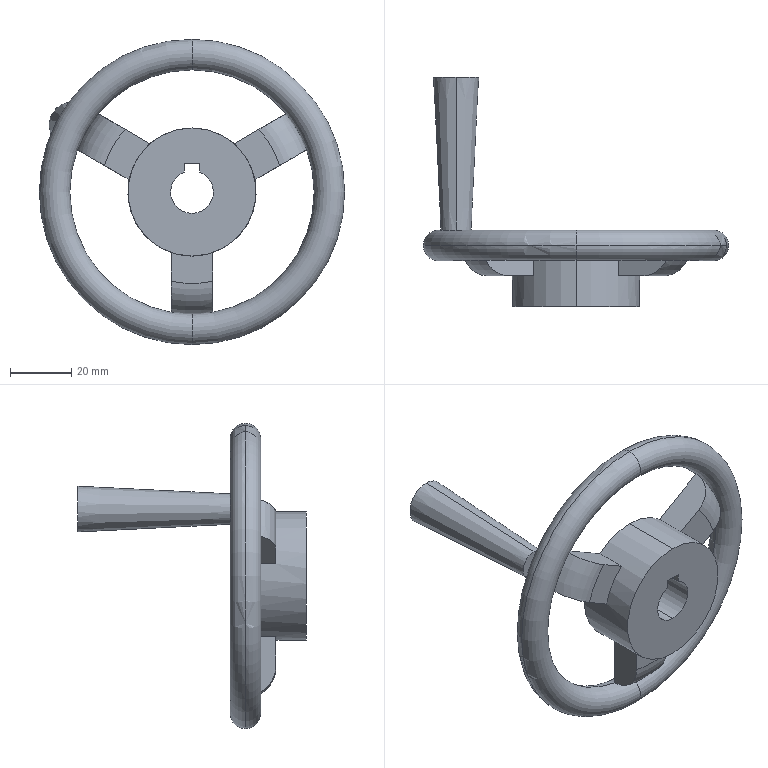Part | SolidWorks | features ICE 4, 3DProfileFeature 1, Fillet 1, Revolution 1, Sweep 1 | 3 solids | 29 faces | box 100 x 75 x 100 mm | volume 59765 mm3 | plane 16 | torus 7 | cylinder 4 | cone 2 | commonest cylinder face diameters 14 x2 42 x2
STEP:
#1=CARTESIAN_POINT('',(0.,0.,-50.));
#2=VERTEX_POINT('',#1);
#3=CARTESIAN_POINT('',(0.,0.,-40.));
#4=VERTEX_POINT('',#3);
#5=CARTESIAN_POINT('',(0.,0.,-45.));
#6=DIRECTION('',(1.,0.,0.));
#7=DIRECTION('',(0.,0.,-1.));
#8=AXIS2_PLACEMENT_3D('',#5,#6,#7);
#9=CIRCLE('',#8,5.);
#10=EDGE_CURVE('',#2,#4,#9,.T.);
#11=ORIENTED_EDGE('',*,*,#10,.F.);
#12=CARTESIAN_POINT('',(0.,0.,50.));
#13=VERTEX_POINT('',#12);
#14=CARTESIAN_POINT('',(0.,0.,0.));
#15=DIRECTION('',(0.,1.,0.));
#16=DIRECTION('',(0.,0.,1.));
#17=AXIS2_PLACEMENT_3D('',#14,#15,#16);
#18=CIRCLE('',#17,50.);
#19=EDGE_CURVE('',#2,#13,#18,.T.);
#20=ORIENTED_EDGE('',*,*,#19,.T.);
#21=CARTESIAN_POINT('',(0.,0.,40.));
#22=VERTEX_POINT('',#21);
#23=CARTESIAN_POINT('',(0.,0.,45.));
#24=DIRECTION('',(-1.,0.,0.));
#25=DIRECTION('',(0.,0.,1.));
#26=AXIS2_PLACEMENT_3D('',#23,#24,#25);
#27=CIRCLE('',#26,5.);
#28=EDGE_CURVE('',#13,#22,#27,.T.);
#29=ORIENTED_EDGE('',*,*,#28,.T.);
#30=CARTESIAN_POINT('',(0.,0.,0.));
#31=DIRECTION('',(0.,1.,0.));
#32=DIRECTION('',(0.,0.,1.));
#33=AXIS2_PLACEMENT_3D('',#30,#31,#32);
#34=CIRCLE('',#33,40.);
#35=EDGE_CURVE('',#4,#22,#34,.T.);
#36=ORIENTED_EDGE('',*,*,#35,.F.);
#37=EDGE_LOOP('',(#11,#20,#29,#36));
#38=FACE_OUTER_BOUND('',#37,.T.);
#39=CARTESIAN_POINT('',(0.,0.,0.));
#40=DIRECTION('',(0.,1.,0.));
#41=DIRECTION('',(0.,0.,1.));
#42=AXIS2_PLACEMENT_3D('',#39,#40,#41);
#43=TOROIDAL_SURFACE('',#42,45.,5.);
#44=ADVANCED_FACE('',(#38),#43,.T.);
#45=ORIENTED_EDGE('',*,*,#28,.F.);
#46=CARTESIAN_POINT('',(0.,0.,0.));
#47=DIRECTION('',(0.,1.,0.));
#48=DIRECTION('',(0.,0.,1.));
#49=AXIS2_PLACEMENT_3D('',#46,#47,#48);
#50=CIRCLE('',#49,50.);
#51=EDGE_CURVE('',#13,#2,#50,.T.);
#52=ORIENTED_EDGE('',*,*,#51,.T.);
#53=ORIENTED_EDGE('',*,*,#10,.T.);
#54=CARTESIAN_POINT('',(0.,0.,0.));
#55=DIRECTION('',(0.,1.,0.));
#56=DIRECTION('',(0.,0.,1.));
#57=AXIS2_PLACEMENT_3D('',#54,#55,#56);
#58=CIRCLE('',#57,40.);
#59=EDGE_CURVE('',#22,#4,#58,.T.);
#60=ORIENTED_EDGE('',*,*,#59,.F.);
#61=EDGE_LOOP('',(#45,#52,#53,#60));
#62=FACE_OUTER_BOUND('',#61,.T.);
#63=CARTESIAN_POINT('',(0.,0.,0.));
#64=DIRECTION('',(0.,1.,0.));
#65=DIRECTION('',(0.,0.,1.));
#66=AXIS2_PLACEMENT_3D('',#63,#64,#65);
#67=TOROIDAL_SURFACE('',#66,45.,5.);
#68=ADVANCED_FACE('',(#62),#67,.T.);
#69=ORIENTED_EDGE('',*,*,#51,.F.);
#70=CARTESIAN_POINT('',(0.,0.,45.));
#71=DIRECTION('',(-1.,0.,0.));
#72=DIRECTION('',(0.,0.,1.));
#73=AXIS2_PLACEMENT_3D('',#70,#71,#72);
#74=CIRCLE('',#73,5.);
#75=EDGE_CURVE('',#22,#13,#74,.T.);
#76=ORIENTED_EDGE('',*,*,#75,.F.);
#77=ORIENTED_EDGE('',*,*,#59,.T.);
#78=CARTESIAN_POINT('',(0.,0.,-45.));
#79=DIRECTION('',(1.,0.,0.));
#80=DIRECTION('',(0.,0.,-1.));
#81=AXIS2_PLACEMENT_3D('',#78,#79,#80);
#82=CIRCLE('',#81,5.);
#83=EDGE_CURVE('',#4,#2,#82,.T.);
#84=ORIENTED_EDGE('',*,*,#83,.T.);
#85=EDGE_LOOP('',(#69,#76,#77,#84));
#86=FACE_OUTER_BOUND('',#85,.T.);
#87=CARTESIAN_POINT('',(0.,0.,0.));
#88=DIRECTION('',(0.,1.,0.));
#89=DIRECTION('',(0.,0.,1.));
#90=AXIS2_PLACEMENT_3D('',#87,#88,#89);
#91=TOROIDAL_SURFACE('',#90,45.,5.);
#92=ADVANCED_FACE('',(#86),#91,.T.);
#93=ORIENTED_EDGE('',*,*,#19,.F.);
#94=ORIENTED_EDGE('',*,*,#83,.F.);
#95=ORIENTED_EDGE('',*,*,#35,.T.);
#96=ORIENTED_EDGE('',*,*,#75,.T.);
#97=EDGE_LOOP('',(#93,#94,#95,#96));
#98=FACE_OUTER_BOUND('',#97,.T.);
#99=CARTESIAN_POINT('',(0.,0.,0.));
#100=DIRECTION('',(0.,1.,0.));
#101=DIRECTION('',(0.,0.,1.));
#102=AXIS2_PLACEMENT_3D('',#99,#100,#101);
#103=TOROIDAL_SURFACE('',#102,45.,5.);
#104=ADVANCED_FACE('',(#98),#103,.T.);
#105=CLOSED_SHELL('',(#44,#68,#92,#104));
#106=MANIFOLD_SOLID_BREP('',#105);
#107=CARTESIAN_POINT('',(-39.297,5.,16.925));
#108=VERTEX_POINT('',#107);
#109=CARTESIAN_POINT('',(-39.297,5.,26.925));
#110=VERTEX_POINT('',#109);
#111=CARTESIAN_POINT('',(-39.297,5.,21.925));
#112=DIRECTION('',(0.,-1.,0.));
#113=DIRECTION('',(0.,0.,-1.));
#114=AXIS2_PLACEMENT_3D('',#111,#112,#113);
#115=CIRCLE('',#114,5.);
#116=EDGE_CURVE('',#108,#110,#115,.T.);
#117=ORIENTED_EDGE('',*,*,#116,.F.);
#118=CARTESIAN_POINT('',(-39.297,55.,14.425));
#119=VERTEX_POINT('',#118);
#120=CARTESIAN_POINT('',(-39.297,55.,14.425));
#121=DIRECTION('',(0.,0.9988,-0.04994));
#122=VECTOR('',#121,1000.);
#123=LINE('',#120,#122);
#124=EDGE_CURVE('',#108,#119,#123,.T.);
#125=ORIENTED_EDGE('',*,*,#124,.T.);
#126=CARTESIAN_POINT('',(-39.297,55.,29.425));
#127=VERTEX_POINT('',#126);
#128=CARTESIAN_POINT('',(-39.297,55.,21.925));
#129=DIRECTION('',(0.,-1.,0.));
#130=DIRECTION('',(0.,0.,-1.));
#131=AXIS2_PLACEMENT_3D('',#128,#129,#130);
#132=CIRCLE('',#131,7.5);
#133=EDGE_CURVE('',#119,#127,#132,.T.);
#134=ORIENTED_EDGE('',*,*,#133,.T.);
#135=CARTESIAN_POINT('',(-39.297,55.,29.425));
#136=DIRECTION('',(0.,0.9988,0.04994));
#137=VECTOR('',#136,1000.);
#138=LINE('',#135,#137);
#139=EDGE_CURVE('',#110,#127,#138,.T.);
#140=ORIENTED_EDGE('',*,*,#139,.F.);
#141=EDGE_LOOP('',(#117,#125,#134,#140));
#142=FACE_OUTER_BOUND('',#141,.T.);
#143=CARTESIAN_POINT('',(-39.297,55.,21.925));
#144=DIRECTION('',(0.,1.,0.));
#145=DIRECTION('',(0.,0.,1.));
#146=AXIS2_PLACEMENT_3D('',#143,#144,#145);
#147=CONICAL_SURFACE('',#146,7.5,0.04996);
#148=ADVANCED_FACE('',(#142),#147,.T.);
#149=ORIENTED_EDGE('',*,*,#124,.F.);
#150=CARTESIAN_POINT('',(-39.297,5.,21.925));
#151=DIRECTION('',(0.,-1.,0.));
#152=DIRECTION('',(0.,0.,-1.));
#153=AXIS2_PLACEMENT_3D('',#150,#151,#152);
#154=CIRCLE('',#153,5.);
#155=EDGE_CURVE('',#110,#108,#154,.T.);
#156=ORIENTED_EDGE('',*,*,#155,.F.);
#157=ORIENTED_EDGE('',*,*,#139,.T.);
#158=CARTESIAN_POINT('',(-39.297,55.,21.925));
#159=DIRECTION('',(0.,-1.,0.));
#160=DIRECTION('',(0.,0.,-1.));
#161=AXIS2_PLACEMENT_3D('',#158,#159,#160);
#162=CIRCLE('',#161,7.5);
#163=EDGE_CURVE('',#127,#119,#162,.T.);
#164=ORIENTED_EDGE('',*,*,#163,.T.);
#165=EDGE_LOOP('',(#149,#156,#157,#164));
#166=FACE_OUTER_BOUND('',#165,.T.);
#167=CARTESIAN_POINT('',(-39.297,55.,21.925));
#168=DIRECTION('',(0.,1.,0.));
#169=DIRECTION('',(0.,0.,1.));
#170=AXIS2_PLACEMENT_3D('',#167,#168,#169);
#171=CONICAL_SURFACE('',#170,7.5,0.04996);
#172=ADVANCED_FACE('',(#166),#171,.T.);
#173=ORIENTED_EDGE('',*,*,#155,.T.);
#174=ORIENTED_EDGE('',*,*,#116,.T.);
#175=EDGE_LOOP('',(#173,#174));
#176=FACE_OUTER_BOUND('',#175,.T.);
#177=CARTESIAN_POINT('',(-39.297,5.,0.));
#178=DIRECTION('',(0.,1.,0.));
#179=DIRECTION('',(0.,0.,1.));
#180=AXIS2_PLACEMENT_3D('',#177,#178,#179);
#181=PLANE('',#180);
#182=ADVANCED_FACE('',(#176),#181,.F.);
#183=ORIENTED_EDGE('',*,*,#163,.F.);
#184=ORIENTED_EDGE('',*,*,#133,.F.);
#185=EDGE_LOOP('',(#183,#184));
#186=FACE_OUTER_BOUND('',#185,.T.);
#187=CARTESIAN_POINT('',(-39.297,55.,0.));
#188=DIRECTION('',(0.,-1.,0.));
#189=DIRECTION('',(0.,0.,-1.));
#190=AXIS2_PLACEMENT_3D('',#187,#188,#189);
#191=PLANE('',#190);
#192=ADVANCED_FACE('',(#186),#191,.F.);
#193=CLOSED_SHELL('',(#148,#172,#182,#192));
#194=MANIFOLD_SOLID_BREP('',#193);
#195=CARTESIAN_POINT('',(2.5,0.,6.538));
#196=VERTEX_POINT('',#195);
#197=CARTESIAN_POINT('',(0.,0.,-7.));
#198=VERTEX_POINT('',#197);
#199=CARTESIAN_POINT('',(0.,0.,0.));
#200=DIRECTION('',(0.,1.,0.));
#201=DIRECTION('',(0.,0.,1.));
#202=AXIS2_PLACEMENT_3D('',#199,#200,#201);
#203=CIRCLE('',#202,7.);
#204=EDGE_CURVE('',#196,#198,#203,.T.);
#205=ORIENTED_EDGE('',*,*,#204,.T.);
#206=CARTESIAN_POINT('',(0.,-20.,-7.));
#207=VERTEX_POINT('',#206);
#208=CARTESIAN_POINT('',(0.,55.,-7.));
#209=DIRECTION('',(0.,-1.,0.));
#210=VECTOR('',#209,1000.);
#211=LINE('',#208,#210);
#212=EDGE_CURVE('',#198,#207,#211,.T.);
#213=ORIENTED_EDGE('',*,*,#212,.T.);
#214=CARTESIAN_POINT('',(2.5,-20.,6.538));
#215=VERTEX_POINT('',#214);
#216=CARTESIAN_POINT('',(0.,-20.,0.));
#217=DIRECTION('',(0.,-1.,0.));
#218=DIRECTION('',(0.,0.,-1.));
#219=AXIS2_PLACEMENT_3D('',#216,#217,#218);
#220=CIRCLE('',#219,7.);
#221=EDGE_CURVE('',#207,#215,#220,.T.);
#222=ORIENTED_EDGE('',*,*,#221,.T.);
#223=CARTESIAN_POINT('',(2.5,55.,6.538));
#224=DIRECTION('',(0.,1.,0.));
#225=VECTOR('',#224,1000.);
#226=LINE('',#223,#225);
#227=EDGE_CURVE('',#215,#196,#226,.T.);
#228=ORIENTED_EDGE('',*,*,#227,.T.);
#229=EDGE_LOOP('',(#205,#213,#222,#228));
#230=FACE_OUTER_BOUND('',#229,.T.);
#231=CARTESIAN_POINT('',(0.,55.,0.));
#232=DIRECTION('',(0.,-1.,0.));
#233=DIRECTION('',(0.,0.,-1.));
#234=AXIS2_PLACEMENT_3D('',#231,#232,#233);
#235=CYLINDRICAL_SURFACE('',#234,7.);
#236=ADVANCED_FACE('',(#230),#235,.F.);
#237=CARTESIAN_POINT('',(0.,-20.,-21.));
#238=VERTEX_POINT('',#237);
#239=CARTESIAN_POINT('',(0.,-20.,21.));
#240=VERTEX_POINT('',#239);
#241=CARTESIAN_POINT('',(0.,-20.,0.));
#242=DIRECTION('',(0.,-1.,0.));
#243=DIRECTION('',(0.,0.,-1.));
#244=AXIS2_PLACEMENT_3D('',#241,#242,#243);
#245=CIRCLE('',#244,21.);
#246=EDGE_CURVE('',#238,#240,#245,.T.);
#247=ORIENTED_EDGE('',*,*,#246,.F.);
#248=CARTESIAN_POINT('',(0.,-10.,-21.));
#249=VERTEX_POINT('',#248);
#250=CARTESIAN_POINT('',(0.,-10.,-21.));
#251=DIRECTION('',(0.,1.,0.));
#252=VECTOR('',#251,1000.);
#253=LINE('',#250,#252);
#254=EDGE_CURVE('',#238,#249,#253,.T.);
#255=ORIENTED_EDGE('',*,*,#254,.T.);
#256=CARTESIAN_POINT('',(6.811,-10.,-19.865));
#257=VERTEX_POINT('',#256);
#258=CARTESIAN_POINT('',(0.,-10.,0.));
#259=DIRECTION('',(0.,-1.,0.));
#260=DIRECTION('',(0.,0.,1.));
#261=AXIS2_PLACEMENT_3D('',#258,#259,#260);
#262=CIRCLE('',#261,21.);
#263=EDGE_CURVE('',#249,#257,#262,.T.);
#264=ORIENTED_EDGE('',*,*,#263,.T.);
#265=CARTESIAN_POINT('',(6.811,0.,-19.865));
#266=VERTEX_POINT('',#265);
#267=CARTESIAN_POINT('',(6.811,-10.,-19.865));
#268=DIRECTION('',(0.,1.,0.));
#269=VECTOR('',#268,1000.);
#270=LINE('',#267,#269);
#271=EDGE_CURVE('',#257,#266,#270,.T.);
#272=ORIENTED_EDGE('',*,*,#271,.T.);
#273=CARTESIAN_POINT('',(20.609,0.,4.034));
#274=VERTEX_POINT('',#273);
#275=CARTESIAN_POINT('',(0.,0.,0.));
#276=DIRECTION('',(0.,1.,0.));
#277=DIRECTION('',(0.,0.,1.));
#278=AXIS2_PLACEMENT_3D('',#275,#276,#277);
#279=CIRCLE('',#278,21.);
#280=EDGE_CURVE('',#274,#266,#279,.T.);
#281=ORIENTED_EDGE('',*,*,#280,.F.);
#282=CARTESIAN_POINT('',(20.609,-10.,4.034));
#283=VERTEX_POINT('',#282);
#284=CARTESIAN_POINT('',(20.609,-10.,4.034));
#285=DIRECTION('',(0.,1.,0.));
#286=VECTOR('',#285,1000.);
#287=LINE('',#284,#286);
#288=EDGE_CURVE('',#283,#274,#287,.T.);
#289=ORIENTED_EDGE('',*,*,#288,.F.);
#290=CARTESIAN_POINT('',(13.798,-10.,15.831));
#291=VERTEX_POINT('',#290);
#292=CARTESIAN_POINT('',(0.,-10.,0.));
#293=DIRECTION('',(0.,-1.,0.));
#294=DIRECTION('',(0.,0.,1.));
#295=AXIS2_PLACEMENT_3D('',#292,#293,#294);
#296=CIRCLE('',#295,21.);
#297=EDGE_CURVE('',#283,#291,#296,.T.);
#298=ORIENTED_EDGE('',*,*,#297,.T.);
#299=CARTESIAN_POINT('',(13.798,0.,15.831));
#300=VERTEX_POINT('',#299);
#301=CARTESIAN_POINT('',(13.798,-10.,15.831));
#302=DIRECTION('',(0.,1.,0.));
#303=VECTOR('',#302,1000.);
#304=LINE('',#301,#303);
#305=EDGE_CURVE('',#291,#300,#304,.T.);
#306=ORIENTED_EDGE('',*,*,#305,.T.);
#307=CARTESIAN_POINT('',(0.,0.,21.));
#308=VERTEX_POINT('',#307);
#309=CARTESIAN_POINT('',(0.,0.,0.));
#310=DIRECTION('',(0.,1.,0.));
#311=DIRECTION('',(0.,0.,1.));
#312=AXIS2_PLACEMENT_3D('',#309,#310,#311);
#313=CIRCLE('',#312,21.);
#314=EDGE_CURVE('',#308,#300,#313,.T.);
#315=ORIENTED_EDGE('',*,*,#314,.F.);
#316=CARTESIAN_POINT('',(0.,-10.,21.));
#317=DIRECTION('',(0.,1.,0.));
#318=VECTOR('',#317,1000.);
#319=LINE('',#316,#318);
#320=EDGE_CURVE('',#240,#308,#319,.T.);
#321=ORIENTED_EDGE('',*,*,#320,.F.);
#322=EDGE_LOOP('',(#247,#255,#264,#272,#281,#289,#298,#306,#315,#321));
#323=FACE_OUTER_BOUND('',#322,.T.);
#324=CARTESIAN_POINT('',(0.,-10.,0.));
#325=DIRECTION('',(0.,1.,0.));
#326=DIRECTION('',(0.,0.,1.));
#327=AXIS2_PLACEMENT_3D('',#324,#325,#326);
#328=CYLINDRICAL_SURFACE('',#327,21.);
#329=ADVANCED_FACE('',(#323),#328,.T.);
#330=CARTESIAN_POINT('',(-13.798,-10.,15.831));
#331=VERTEX_POINT('',#330);
#332=CARTESIAN_POINT('',(-20.609,-10.,4.034));
#333=VERTEX_POINT('',#332);
#334=CARTESIAN_POINT('',(0.,-10.,0.));
#335=DIRECTION('',(0.,-1.,0.));
#336=DIRECTION('',(0.,0.,1.));
#337=AXIS2_PLACEMENT_3D('',#334,#335,#336);
#338=CIRCLE('',#337,21.);
#339=EDGE_CURVE('',#331,#333,#338,.T.);
#340=ORIENTED_EDGE('',*,*,#339,.F.);
#341=CARTESIAN_POINT('',(-21.897,-10.,20.507));
#342=VERTEX_POINT('',#341);
#343=CARTESIAN_POINT('',(3.405,-10.,5.898));
#344=DIRECTION('',(-0.866,0.,0.5));
#345=VECTOR('',#344,1000.);
#346=LINE('',#343,#345);
#347=EDGE_CURVE('',#331,#342,#346,.T.);
#348=ORIENTED_EDGE('',*,*,#347,.T.);
#349=CARTESIAN_POINT('',(-28.708,-10.,8.71));
#350=VERTEX_POINT('',#349);
#351=CARTESIAN_POINT('',(0.,-10.,0.));
#352=DIRECTION('',(0.,-1.,0.));
#353=DIRECTION('',(0.,0.,1.));
#354=AXIS2_PLACEMENT_3D('',#351,#352,#353);
#355=CIRCLE('',#354,30.);
#356=EDGE_CURVE('',#342,#350,#355,.T.);
#357=ORIENTED_EDGE('',*,*,#356,.T.);
#358=CARTESIAN_POINT('',(-3.405,-10.,-5.898));
#359=DIRECTION('',(-0.866,0.,0.5));
#360=VECTOR('',#359,1000.);
#361=LINE('',#358,#360);
#362=EDGE_CURVE('',#333,#350,#361,.T.);
#363=ORIENTED_EDGE('',*,*,#362,.F.);
#364=EDGE_LOOP('',(#340,#348,#357,#363));
#365=FACE_OUTER_BOUND('',#364,.T.);
#366=CARTESIAN_POINT('',(0.,-10.,0.));
#367=DIRECTION('',(0.,1.,0.));
#368=DIRECTION('',(0.,0.,1.));
#369=AXIS2_PLACEMENT_3D('',#366,#367,#368);
#370=PLANE('',#369);
#371=ADVANCED_FACE('',(#365),#370,.F.);
#372=CARTESIAN_POINT('',(-6.811,-10.,-19.865));
#373=VERTEX_POINT('',#372);
#374=CARTESIAN_POINT('',(0.,-10.,0.));
#375=DIRECTION('',(0.,-1.,0.));
#376=DIRECTION('',(0.,0.,1.));
#377=AXIS2_PLACEMENT_3D('',#374,#375,#376);
#378=CIRCLE('',#377,21.);
#379=EDGE_CURVE('',#373,#249,#378,.T.);
#380=ORIENTED_EDGE('',*,*,#379,.F.);
#381=CARTESIAN_POINT('',(-6.811,-10.,-29.217));
#382=VERTEX_POINT('',#381);
#383=CARTESIAN_POINT('',(-6.811,-10.,0.));
#384=DIRECTION('',(0.,0.,-1.));
#385=VECTOR('',#384,1000.);
#386=LINE('',#383,#385);
#387=EDGE_CURVE('',#373,#382,#386,.T.);
#388=ORIENTED_EDGE('',*,*,#387,.T.);
#389=CARTESIAN_POINT('',(6.811,-10.,-29.217));
#390=VERTEX_POINT('',#389);
#391=CARTESIAN_POINT('',(0.,-10.,0.));
#392=DIRECTION('',(0.,-1.,0.));
#393=DIRECTION('',(0.,0.,1.));
#394=AXIS2_PLACEMENT_3D('',#391,#392,#393);
#395=CIRCLE('',#394,30.);
#396=EDGE_CURVE('',#382,#390,#395,.T.);
#397=ORIENTED_EDGE('',*,*,#396,.T.);
#398=CARTESIAN_POINT('',(6.811,-10.,0.));
#399=DIRECTION('',(0.,0.,-1.));
#400=VECTOR('',#399,1000.);
#401=LINE('',#398,#400);
#402=EDGE_CURVE('',#257,#390,#401,.T.);
#403=ORIENTED_EDGE('',*,*,#402,.F.);
#404=ORIENTED_EDGE('',*,*,#263,.F.);
#405=EDGE_LOOP('',(#380,#388,#397,#403,#404));
#406=FACE_OUTER_BOUND('',#405,.T.);
#407=CARTESIAN_POINT('',(0.,-10.,0.));
#408=DIRECTION('',(0.,1.,0.));
#409=DIRECTION('',(0.,0.,1.));
#410=AXIS2_PLACEMENT_3D('',#407,#408,#409);
#411=PLANE('',#410);
#412=ADVANCED_FACE('',(#406),#411,.F.);
#413=ORIENTED_EDGE('',*,*,#297,.F.);
#414=CARTESIAN_POINT('',(28.708,-10.,8.71));
#415=VERTEX_POINT('',#414);
#416=CARTESIAN_POINT('',(3.405,-10.,-5.898));
#417=DIRECTION('',(0.866,0.,0.5));
#418=VECTOR('',#417,1000.);
#419=LINE('',#416,#418);
#420=EDGE_CURVE('',#283,#415,#419,.T.);
#421=ORIENTED_EDGE('',*,*,#420,.T.);
#422=CARTESIAN_POINT('',(21.897,-10.,20.507));
#423=VERTEX_POINT('',#422);
#424=CARTESIAN_POINT('',(0.,-10.,0.));
#425=DIRECTION('',(0.,-1.,0.));
#426=DIRECTION('',(0.,0.,1.));
#427=AXIS2_PLACEMENT_3D('',#424,#425,#426);
#428=CIRCLE('',#427,30.);
#429=EDGE_CURVE('',#415,#423,#428,.T.);
#430=ORIENTED_EDGE('',*,*,#429,.T.);
#431=CARTESIAN_POINT('',(-3.405,-10.,5.898));
#432=DIRECTION('',(0.866,0.,0.5));
#433=VECTOR('',#432,1000.);
#434=LINE('',#431,#433);
#435=EDGE_CURVE('',#291,#423,#434,.T.);
#436=ORIENTED_EDGE('',*,*,#435,.F.);
#437=EDGE_LOOP('',(#413,#421,#430,#436));
#438=FACE_OUTER_BOUND('',#437,.T.);
#439=CARTESIAN_POINT('',(0.,-10.,0.));
#440=DIRECTION('',(0.,1.,0.));
#441=DIRECTION('',(0.,0.,1.));
#442=AXIS2_PLACEMENT_3D('',#439,#440,#441);
#443=PLANE('',#442);
#444=ADVANCED_FACE('',(#438),#443,.F.);
#445=ORIENTED_EDGE('',*,*,#402,.T.);
#446=CARTESIAN_POINT('',(6.811,0.,-39.416));
#447=VERTEX_POINT('',#446);
#448=CARTESIAN_POINT('',(6.811,-10.,-29.217));
#449=CARTESIAN_POINT('',(6.811,-10.,-29.884));
#450=CARTESIAN_POINT('',(6.811,-9.937,-30.54));
#451=CARTESIAN_POINT('',(6.811,-9.752,-31.509));
#452=CARTESIAN_POINT('',(6.811,-9.675,-31.83));
#453=CARTESIAN_POINT('',(6.811,-9.489,-32.465));
#454=CARTESIAN_POINT('',(6.811,-9.38,-32.782));
#455=CARTESIAN_POINT('',(6.811,-9.01,-33.705));
#456=CARTESIAN_POINT('',(6.811,-8.708,-34.289));
#457=CARTESIAN_POINT('',(6.811,-7.993,-35.396));
#458=CARTESIAN_POINT('',(6.811,-7.574,-35.922));
#459=CARTESIAN_POINT('',(6.811,-6.655,-36.869));
#460=CARTESIAN_POINT('',(6.811,-6.153,-37.293));
#461=CARTESIAN_POINT('',(6.811,-5.335,-37.856));
#462=CARTESIAN_POINT('',(6.811,-5.05,-38.032));
#463=CARTESIAN_POINT('',(6.811,-4.469,-38.352));
#464=CARTESIAN_POINT('',(6.811,-4.173,-38.496));
#465=CARTESIAN_POINT('',(6.811,-3.265,-38.883));
#466=CARTESIAN_POINT('',(6.811,-2.635,-39.081));
#467=CARTESIAN_POINT('',(6.811,-1.328,-39.349));
#468=CARTESIAN_POINT('',(6.811,-0.6674,-39.416));
#469=CARTESIAN_POINT('',(6.811,0.,-39.416));
#470=B_SPLINE_CURVE_WITH_KNOTS('',3,(#448,#449,#450,#451,#452,#453,#454,#455,#456,#457,#458,#459,#460,#461,#462,#463,#464,#465,#466,#467,#468,#469),.UNSPECIFIED.,.F.,.F.,(4,2,2,2,2,2,2,2,2,2,4),(0.,0.001973,0.00296,0.003946,0.005919,0.007892,0.009865,0.01085,0.01184,0.01381,0.01578),.UNSPECIFIED.);
#471=EDGE_CURVE('',#390,#447,#470,.T.);
#472=ORIENTED_EDGE('',*,*,#471,.T.);
#473=CARTESIAN_POINT('',(6.811,0.,0.));
#474=DIRECTION('',(0.,0.,-1.));
#475=VECTOR('',#474,1000.);
#476=LINE('',#473,#475);
#477=EDGE_CURVE('',#266,#447,#476,.T.);
#478=ORIENTED_EDGE('',*,*,#477,.F.);
#479=ORIENTED_EDGE('',*,*,#271,.F.);
#480=EDGE_LOOP('',(#445,#472,#478,#479));
#481=FACE_OUTER_BOUND('',#480,.T.);
#482=CARTESIAN_POINT('',(6.811,-10.,0.));
#483=DIRECTION('',(1.,0.,0.));
#484=DIRECTION('',(0.,0.,-1.));
#485=AXIS2_PLACEMENT_3D('',#482,#483,#484);
#486=PLANE('',#485);
#487=ADVANCED_FACE('',(#481),#486,.T.);
#488=ORIENTED_EDGE('',*,*,#254,.F.);
#489=CARTESIAN_POINT('',(0.,-20.,0.));
#490=DIRECTION('',(0.,-1.,0.));
#491=DIRECTION('',(0.,0.,-1.));
#492=AXIS2_PLACEMENT_3D('',#489,#490,#491);
#493=CIRCLE('',#492,21.);
#494=EDGE_CURVE('',#240,#238,#493,.T.);
#495=ORIENTED_EDGE('',*,*,#494,.F.);
#496=ORIENTED_EDGE('',*,*,#320,.T.);
#497=CARTESIAN_POINT('',(-13.798,0.,15.831));
#498=VERTEX_POINT('',#497);
#499=CARTESIAN_POINT('',(0.,0.,0.));
#500=DIRECTION('',(0.,1.,0.));
#501=DIRECTION('',(0.,0.,1.));
#502=AXIS2_PLACEMENT_3D('',#499,#500,#501);
#503=CIRCLE('',#502,21.);
#504=EDGE_CURVE('',#498,#308,#503,.T.);
#505=ORIENTED_EDGE('',*,*,#504,.F.);
#506=CARTESIAN_POINT('',(-13.798,-10.,15.831));
#507=DIRECTION('',(0.,1.,0.));
#508=VECTOR('',#507,1000.);
#509=LINE('',#506,#508);
#510=EDGE_CURVE('',#331,#498,#509,.T.);
#511=ORIENTED_EDGE('',*,*,#510,.F.);
#512=ORIENTED_EDGE('',*,*,#339,.T.);
#513=CARTESIAN_POINT('',(-20.609,0.,4.034));
#514=VERTEX_POINT('',#513);
#515=CARTESIAN_POINT('',(-20.609,-10.,4.034));
#516=DIRECTION('',(0.,1.,0.));
#517=VECTOR('',#516,1000.);
#518=LINE('',#515,#517);
#519=EDGE_CURVE('',#333,#514,#518,.T.);
#520=ORIENTED_EDGE('',*,*,#519,.T.);
#521=CARTESIAN_POINT('',(-6.811,0.,-19.865));
#522=VERTEX_POINT('',#521);
#523=CARTESIAN_POINT('',(0.,0.,0.));
#524=DIRECTION('',(0.,1.,0.));
#525=DIRECTION('',(0.,0.,1.));
#526=AXIS2_PLACEMENT_3D('',#523,#524,#525);
#527=CIRCLE('',#526,21.);
#528=EDGE_CURVE('',#522,#514,#527,.T.);
#529=ORIENTED_EDGE('',*,*,#528,.F.);
#530=CARTESIAN_POINT('',(-6.811,-10.,-19.865));
#531=DIRECTION('',(0.,1.,0.));
#532=VECTOR('',#531,1000.);
#533=LINE('',#530,#532);
#534=EDGE_CURVE('',#373,#522,#533,.T.);
#535=ORIENTED_EDGE('',*,*,#534,.F.);
#536=ORIENTED_EDGE('',*,*,#379,.T.);
#537=EDGE_LOOP('',(#488,#495,#496,#505,#511,#512,#520,#529,#535,#536));
#538=FACE_OUTER_BOUND('',#537,.T.);
#539=CARTESIAN_POINT('',(0.,-10.,0.));
#540=DIRECTION('',(0.,1.,0.));
#541=DIRECTION('',(0.,0.,1.));
#542=AXIS2_PLACEMENT_3D('',#539,#540,#541);
#543=CYLINDRICAL_SURFACE('',#542,21.);
#544=ADVANCED_FACE('',(#538),#543,.T.);
#545=CARTESIAN_POINT('',(37.541,0.,13.81));
#546=VERTEX_POINT('',#545);
#547=CARTESIAN_POINT('',(3.405,0.,-5.898));
#548=DIRECTION('',(0.866,0.,0.5));
#549=VECTOR('',#548,1000.);
#550=LINE('',#547,#549);
#551=EDGE_CURVE('',#274,#546,#550,.T.);
#552=ORIENTED_EDGE('',*,*,#551,.T.);
#553=CARTESIAN_POINT('',(37.541,0.,13.81));
#554=CARTESIAN_POINT('',(37.541,-0.6672,13.81));
#555=CARTESIAN_POINT('',(37.482,-1.323,13.776));
#556=CARTESIAN_POINT('',(37.312,-2.29,13.678));
#557=CARTESIAN_POINT('',(37.241,-2.61,13.637));
#558=CARTESIAN_POINT('',(37.071,-3.243,13.538));
#559=CARTESIAN_POINT('',(36.971,-3.558,13.481));
#560=CARTESIAN_POINT('',(36.635,-4.47,13.286));
#561=CARTESIAN_POINT('',(36.36,-5.047,13.128));
#562=CARTESIAN_POINT('',(35.875,-5.865,12.848));
#563=CARTESIAN_POINT('',(35.7,-6.131,12.747));
#564=CARTESIAN_POINT('',(35.329,-6.638,12.533));
#565=CARTESIAN_POINT('',(35.134,-6.88,12.42));
#566=CARTESIAN_POINT('',(34.521,-7.568,12.066));
#567=CARTESIAN_POINT('',(34.075,-7.98,11.809));
#568=CARTESIAN_POINT('',(33.107,-8.704,11.25));
#569=CARTESIAN_POINT('',(32.598,-9.008,10.956));
#570=CARTESIAN_POINT('',(31.805,-9.376,10.498));
#571=CARTESIAN_POINT('',(31.535,-9.484,10.342));
#572=CARTESIAN_POINT('',(30.985,-9.671,10.025));
#573=CARTESIAN_POINT('',(30.703,-9.749,9.862));
#574=CARTESIAN_POINT('',(29.856,-9.937,9.373));
#575=CARTESIAN_POINT('',(29.285,-10.,9.043));
#576=CARTESIAN_POINT('',(28.708,-10.,8.71));
#577=B_SPLINE_CURVE_WITH_KNOTS('',3,(#553,#554,#555,#556,#557,#558,#559,#560,#561,#562,#563,#564,#565,#566,#567,#568,#569,#570,#571,#572,#573,#574,#575,#576),.UNSPECIFIED.,.F.,.F.,(4,2,2,2,2,2,2,2,2,2,2,4),(0.,0.001973,0.00296,0.003946,0.005919,0.006906,0.007892,0.009865,0.01184,0.01282,0.01381,0.01578),.UNSPECIFIED.);
#578=EDGE_CURVE('',#546,#415,#577,.T.);
#579=ORIENTED_EDGE('',*,*,#578,.T.);
#580=ORIENTED_EDGE('',*,*,#420,.F.);
#581=ORIENTED_EDGE('',*,*,#288,.T.);
#582=EDGE_LOOP('',(#552,#579,#580,#581));
#583=FACE_OUTER_BOUND('',#582,.T.);
#584=CARTESIAN_POINT('',(3.405,-10.,-5.898));
#585=DIRECTION('',(-0.5,0.,0.866));
#586=DIRECTION('',(0.866,0.,0.5));
#587=AXIS2_PLACEMENT_3D('',#584,#585,#586);
#588=PLANE('',#587);
#589=ADVANCED_FACE('',(#583),#588,.F.);
#590=ORIENTED_EDGE('',*,*,#435,.T.);
#591=CARTESIAN_POINT('',(30.73,0.,25.606));
#592=VERTEX_POINT('',#591);
#593=CARTESIAN_POINT('',(21.897,-10.,20.507));
#594=CARTESIAN_POINT('',(22.475,-10.,20.84));
#595=CARTESIAN_POINT('',(23.043,-9.937,21.168));
#596=CARTESIAN_POINT('',(23.882,-9.752,21.653));
#597=CARTESIAN_POINT('',(24.16,-9.675,21.813));
#598=CARTESIAN_POINT('',(24.71,-9.489,22.131));
#599=CARTESIAN_POINT('',(24.985,-9.38,22.289));
#600=CARTESIAN_POINT('',(25.784,-9.01,22.751));
#601=CARTESIAN_POINT('',(26.29,-8.708,23.043));
#602=CARTESIAN_POINT('',(27.248,-7.993,23.596));
#603=CARTESIAN_POINT('',(27.704,-7.574,23.859));
#604=CARTESIAN_POINT('',(28.524,-6.655,24.333));
#605=CARTESIAN_POINT('',(28.892,-6.153,24.545));
#606=CARTESIAN_POINT('',(29.379,-5.335,24.827));
#607=CARTESIAN_POINT('',(29.532,-5.05,24.915));
#608=CARTESIAN_POINT('',(29.808,-4.469,25.074));
#609=CARTESIAN_POINT('',(29.933,-4.173,25.146));
#610=CARTESIAN_POINT('',(30.268,-3.265,25.34));
#611=CARTESIAN_POINT('',(30.439,-2.635,25.439));
#612=CARTESIAN_POINT('',(30.672,-1.328,25.573));
#613=CARTESIAN_POINT('',(30.73,-0.6674,25.606));
#614=CARTESIAN_POINT('',(30.73,0.,25.606));
#615=B_SPLINE_CURVE_WITH_KNOTS('',3,(#593,#594,#595,#596,#597,#598,#599,#600,#601,#602,#603,#604,#605,#606,#607,#608,#609,#610,#611,#612,#613,#614),.UNSPECIFIED.,.F.,.F.,(4,2,2,2,2,2,2,2,2,2,4),(0.,0.001973,0.00296,0.003946,0.005919,0.007892,0.009865,0.01085,0.01184,0.01381,0.01578),.UNSPECIFIED.);
#616=EDGE_CURVE('',#423,#592,#615,.T.);
#617=ORIENTED_EDGE('',*,*,#616,.T.);
#618=CARTESIAN_POINT('',(-3.405,0.,5.898));
#619=DIRECTION('',(0.866,0.,0.5));
#620=VECTOR('',#619,1000.);
#621=LINE('',#618,#620);
#622=EDGE_CURVE('',#300,#592,#621,.T.);
#623=ORIENTED_EDGE('',*,*,#622,.F.);
#624=ORIENTED_EDGE('',*,*,#305,.F.);
#625=EDGE_LOOP('',(#590,#617,#623,#624));
#626=FACE_OUTER_BOUND('',#625,.T.);
#627=CARTESIAN_POINT('',(-3.405,-10.,5.898));
#628=DIRECTION('',(-0.5,0.,0.866));
#629=DIRECTION('',(0.866,0.,0.5));
#630=AXIS2_PLACEMENT_3D('',#627,#628,#629);
#631=PLANE('',#630);
#632=ADVANCED_FACE('',(#626),#631,.T.);
#633=CARTESIAN_POINT('',(-30.73,0.,25.606));
#634=VERTEX_POINT('',#633);
#635=CARTESIAN_POINT('',(3.405,0.,5.898));
#636=DIRECTION('',(-0.866,0.,0.5));
#637=VECTOR('',#636,1000.);
#638=LINE('',#635,#637);
#639=EDGE_CURVE('',#498,#634,#638,.T.);
#640=ORIENTED_EDGE('',*,*,#639,.T.);
#641=CARTESIAN_POINT('',(-30.73,0.,25.606));
#642=CARTESIAN_POINT('',(-30.73,-0.6672,25.606));
#643=CARTESIAN_POINT('',(-30.672,-1.323,25.573));
#644=CARTESIAN_POINT('',(-30.501,-2.29,25.474));
#645=CARTESIAN_POINT('',(-30.43,-2.61,25.433));
#646=CARTESIAN_POINT('',(-30.26,-3.243,25.335));
#647=CARTESIAN_POINT('',(-30.16,-3.558,25.277));
#648=CARTESIAN_POINT('',(-29.824,-4.47,25.083));
#649=CARTESIAN_POINT('',(-29.55,-5.047,24.925));
#650=CARTESIAN_POINT('',(-29.064,-5.865,24.645));
#651=CARTESIAN_POINT('',(-28.889,-6.131,24.544));
#652=CARTESIAN_POINT('',(-28.518,-6.638,24.329));
#653=CARTESIAN_POINT('',(-28.323,-6.88,24.217));
#654=CARTESIAN_POINT('',(-27.71,-7.568,23.863));
#655=CARTESIAN_POINT('',(-27.264,-7.98,23.605));
#656=CARTESIAN_POINT('',(-26.297,-8.704,23.047));
#657=CARTESIAN_POINT('',(-25.787,-9.008,22.753));
#658=CARTESIAN_POINT('',(-24.994,-9.376,22.295));
#659=CARTESIAN_POINT('',(-24.724,-9.484,22.139));
#660=CARTESIAN_POINT('',(-24.174,-9.671,21.821));
#661=CARTESIAN_POINT('',(-23.893,-9.749,21.659));
#662=CARTESIAN_POINT('',(-23.046,-9.937,21.17));
#663=CARTESIAN_POINT('',(-22.474,-10.,20.84));
#664=CARTESIAN_POINT('',(-21.897,-10.,20.507));
#665=B_SPLINE_CURVE_WITH_KNOTS('',3,(#641,#642,#643,#644,#645,#646,#647,#648,#649,#650,#651,#652,#653,#654,#655,#656,#657,#658,#659,#660,#661,#662,#663,#664),.UNSPECIFIED.,.F.,.F.,(4,2,2,2,2,2,2,2,2,2,2,4),(0.,0.001973,0.00296,0.003946,0.005919,0.006906,0.007892,0.009865,0.01184,0.01282,0.01381,0.01578),.UNSPECIFIED.);
#666=EDGE_CURVE('',#634,#342,#665,.T.);
#667=ORIENTED_EDGE('',*,*,#666,.T.);
#668=ORIENTED_EDGE('',*,*,#347,.F.);
#669=ORIENTED_EDGE('',*,*,#510,.T.);
#670=EDGE_LOOP('',(#640,#667,#668,#669));
#671=FACE_OUTER_BOUND('',#670,.T.);
#672=CARTESIAN_POINT('',(3.405,-10.,5.898));
#673=DIRECTION('',(-0.5,0.,-0.866));
#674=DIRECTION('',(-0.866,0.,0.5));
#675=AXIS2_PLACEMENT_3D('',#672,#673,#674);
#676=PLANE('',#675);
#677=ADVANCED_FACE('',(#671),#676,.F.);
#678=ORIENTED_EDGE('',*,*,#362,.T.);
#679=CARTESIAN_POINT('',(-37.541,0.,13.81));
#680=VERTEX_POINT('',#679);
#681=CARTESIAN_POINT('',(-28.708,-10.,8.71));
#682=CARTESIAN_POINT('',(-29.285,-10.,9.043));
#683=CARTESIAN_POINT('',(-29.854,-9.937,9.372));
#684=CARTESIAN_POINT('',(-30.693,-9.752,9.856));
#685=CARTESIAN_POINT('',(-30.971,-9.675,10.016));
#686=CARTESIAN_POINT('',(-31.521,-9.489,10.334));
#687=CARTESIAN_POINT('',(-31.795,-9.38,10.493));
#688=CARTESIAN_POINT('',(-32.595,-9.01,10.954));
#689=CARTESIAN_POINT('',(-33.1,-8.708,11.246));
#690=CARTESIAN_POINT('',(-34.059,-7.993,11.799));
#691=CARTESIAN_POINT('',(-34.515,-7.574,12.063));
#692=CARTESIAN_POINT('',(-35.335,-6.655,12.536));
#693=CARTESIAN_POINT('',(-35.702,-6.153,12.748));
#694=CARTESIAN_POINT('',(-36.19,-5.335,13.03));
#695=CARTESIAN_POINT('',(-36.342,-5.05,13.118));
#696=CARTESIAN_POINT('',(-36.619,-4.469,13.277));
#697=CARTESIAN_POINT('',(-36.744,-4.173,13.35));
#698=CARTESIAN_POINT('',(-37.079,-3.265,13.543));
#699=CARTESIAN_POINT('',(-37.25,-2.635,13.642));
#700=CARTESIAN_POINT('',(-37.482,-1.328,13.776));
#701=CARTESIAN_POINT('',(-37.541,-0.6674,13.81));
#702=CARTESIAN_POINT('',(-37.541,0.,13.81));
#703=B_SPLINE_CURVE_WITH_KNOTS('',3,(#681,#682,#683,#684,#685,#686,#687,#688,#689,#690,#691,#692,#693,#694,#695,#696,#697,#698,#699,#700,#701,#702),.UNSPECIFIED.,.F.,.F.,(4,2,2,2,2,2,2,2,2,2,4),(0.,0.001973,0.00296,0.003946,0.005919,0.007892,0.009865,0.01085,0.01184,0.01381,0.01578),.UNSPECIFIED.);
#704=EDGE_CURVE('',#350,#680,#703,.T.);
#705=ORIENTED_EDGE('',*,*,#704,.T.);
#706=CARTESIAN_POINT('',(-3.405,0.,-5.898));
#707=DIRECTION('',(-0.866,0.,0.5));
#708=VECTOR('',#707,1000.);
#709=LINE('',#706,#708);
#710=EDGE_CURVE('',#514,#680,#709,.T.);
#711=ORIENTED_EDGE('',*,*,#710,.F.);
#712=ORIENTED_EDGE('',*,*,#519,.F.);
#713=EDGE_LOOP('',(#678,#705,#711,#712));
#714=FACE_OUTER_BOUND('',#713,.T.);
#715=CARTESIAN_POINT('',(-3.405,-10.,-5.898));
#716=DIRECTION('',(-0.5,0.,-0.866));
#717=DIRECTION('',(-0.866,0.,0.5));
#718=AXIS2_PLACEMENT_3D('',#715,#716,#717);
#719=PLANE('',#718);
#720=ADVANCED_FACE('',(#714),#719,.T.);
#721=CARTESIAN_POINT('',(-6.811,0.,-39.416));
#722=VERTEX_POINT('',#721);
#723=CARTESIAN_POINT('',(-6.811,0.,0.));
#724=DIRECTION('',(0.,0.,-1.));
#725=VECTOR('',#724,1000.);
#726=LINE('',#723,#725);
#727=EDGE_CURVE('',#522,#722,#726,.T.);
#728=ORIENTED_EDGE('',*,*,#727,.T.);
#729=CARTESIAN_POINT('',(-6.811,0.,-39.416));
#730=CARTESIAN_POINT('',(-6.811,-0.6672,-39.416));
#731=CARTESIAN_POINT('',(-6.811,-1.323,-39.349));
#732=CARTESIAN_POINT('',(-6.811,-2.29,-39.152));
#733=CARTESIAN_POINT('',(-6.811,-2.61,-39.07));
#734=CARTESIAN_POINT('',(-6.811,-3.243,-38.873));
#735=CARTESIAN_POINT('',(-6.811,-3.558,-38.758));
#736=CARTESIAN_POINT('',(-6.811,-4.47,-38.37));
#737=CARTESIAN_POINT('',(-6.811,-5.047,-38.053));
#738=CARTESIAN_POINT('',(-6.811,-5.865,-37.493));
#739=CARTESIAN_POINT('',(-6.811,-6.131,-37.29));
#740=CARTESIAN_POINT('',(-6.811,-6.638,-36.862));
#741=CARTESIAN_POINT('',(-6.811,-6.88,-36.637));
#742=CARTESIAN_POINT('',(-6.811,-7.568,-35.929));
#743=CARTESIAN_POINT('',(-6.811,-7.98,-35.414));
#744=CARTESIAN_POINT('',(-6.811,-8.704,-34.297));
#745=CARTESIAN_POINT('',(-6.811,-9.008,-33.709));
#746=CARTESIAN_POINT('',(-6.811,-9.376,-32.793));
#747=CARTESIAN_POINT('',(-6.811,-9.484,-32.481));
#748=CARTESIAN_POINT('',(-6.811,-9.671,-31.846));
#749=CARTESIAN_POINT('',(-6.811,-9.749,-31.521));
#750=CARTESIAN_POINT('',(-6.811,-9.937,-30.543));
#751=CARTESIAN_POINT('',(-6.811,-10.,-29.883));
#752=CARTESIAN_POINT('',(-6.811,-10.,-29.217));
#753=B_SPLINE_CURVE_WITH_KNOTS('',3,(#729,#730,#731,#732,#733,#734,#735,#736,#737,#738,#739,#740,#741,#742,#743,#744,#745,#746,#747,#748,#749,#750,#751,#752),.UNSPECIFIED.,.F.,.F.,(4,2,2,2,2,2,2,2,2,2,2,4),(0.,0.001973,0.00296,0.003946,0.005919,0.006906,0.007892,0.009865,0.01184,0.01282,0.01381,0.01578),.UNSPECIFIED.);
#754=EDGE_CURVE('',#722,#382,#753,.T.);
#755=ORIENTED_EDGE('',*,*,#754,.T.);
#756=ORIENTED_EDGE('',*,*,#387,.F.);
#757=ORIENTED_EDGE('',*,*,#534,.T.);
#758=EDGE_LOOP('',(#728,#755,#756,#757));
#759=FACE_OUTER_BOUND('',#758,.T.);
#760=CARTESIAN_POINT('',(-6.811,-10.,0.));
#761=DIRECTION('',(1.,0.,0.));
#762=DIRECTION('',(0.,0.,-1.));
#763=AXIS2_PLACEMENT_3D('',#760,#761,#762);
#764=PLANE('',#763);
#765=ADVANCED_FACE('',(#759),#764,.F.);
#766=CARTESIAN_POINT('',(2.5,0.,9.3));
#767=VERTEX_POINT('',#766);
#768=CARTESIAN_POINT('',(2.5,0.,0.));
#769=DIRECTION('',(0.,0.,-1.));
#770=VECTOR('',#769,1000.);
#771=LINE('',#768,#770);
#772=EDGE_CURVE('',#767,#196,#771,.T.);
#773=ORIENTED_EDGE('',*,*,#772,.F.);
#774=CARTESIAN_POINT('',(-2.5,0.,9.3));
#775=VERTEX_POINT('',#774);
#776=CARTESIAN_POINT('',(0.,0.,9.3));
#777=DIRECTION('',(1.,0.,0.));
#778=VECTOR('',#777,1000.);
#779=LINE('',#776,#778);
#780=EDGE_CURVE('',#775,#767,#779,.T.);
#781=ORIENTED_EDGE('',*,*,#780,.F.);
#782=CARTESIAN_POINT('',(-2.5,0.,6.538));
#783=VERTEX_POINT('',#782);
#784=CARTESIAN_POINT('',(-2.5,0.,0.));
#785=DIRECTION('',(0.,0.,1.));
#786=VECTOR('',#785,1000.);
#787=LINE('',#784,#786);
#788=EDGE_CURVE('',#783,#775,#787,.T.);
#789=ORIENTED_EDGE('',*,*,#788,.F.);
#790=CARTESIAN_POINT('',(0.,0.,0.));
#791=DIRECTION('',(0.,1.,0.));
#792=DIRECTION('',(0.,0.,1.));
#793=AXIS2_PLACEMENT_3D('',#790,#791,#792);
#794=CIRCLE('',#793,7.);
#795=EDGE_CURVE('',#198,#783,#794,.T.);
#796=ORIENTED_EDGE('',*,*,#795,.F.);
#797=ORIENTED_EDGE('',*,*,#204,.F.);
#798=EDGE_LOOP('',(#773,#781,#789,#796,#797));
#799=FACE_BOUND('',#798,.T.);
#800=CARTESIAN_POINT('',(0.,0.,0.));
#801=DIRECTION('',(0.,1.,0.));
#802=DIRECTION('',(0.,0.,1.));
#803=AXIS2_PLACEMENT_3D('',#800,#801,#802);
#804=CIRCLE('',#803,40.);
#805=EDGE_CURVE('',#447,#722,#804,.T.);
#806=ORIENTED_EDGE('',*,*,#805,.T.);
#807=ORIENTED_EDGE('',*,*,#727,.F.);
#808=ORIENTED_EDGE('',*,*,#528,.T.);
#809=ORIENTED_EDGE('',*,*,#710,.T.);
#810=CARTESIAN_POINT('',(0.,0.,0.));
#811=DIRECTION('',(0.,1.,0.));
#812=DIRECTION('',(0.,0.,1.));
#813=AXIS2_PLACEMENT_3D('',#810,#811,#812);
#814=CIRCLE('',#813,40.);
#815=EDGE_CURVE('',#680,#634,#814,.T.);
#816=ORIENTED_EDGE('',*,*,#815,.T.);
#817=ORIENTED_EDGE('',*,*,#639,.F.);
#818=ORIENTED_EDGE('',*,*,#504,.T.);
#819=ORIENTED_EDGE('',*,*,#314,.T.);
#820=ORIENTED_EDGE('',*,*,#622,.T.);
#821=CARTESIAN_POINT('',(0.,0.,0.));
#822=DIRECTION('',(0.,1.,0.));
#823=DIRECTION('',(0.,0.,1.));
#824=AXIS2_PLACEMENT_3D('',#821,#822,#823);
#825=CIRCLE('',#824,40.);
#826=EDGE_CURVE('',#592,#546,#825,.T.);
#827=ORIENTED_EDGE('',*,*,#826,.T.);
#828=ORIENTED_EDGE('',*,*,#551,.F.);
#829=ORIENTED_EDGE('',*,*,#280,.T.);
#830=ORIENTED_EDGE('',*,*,#477,.T.);
#831=EDGE_LOOP('',(#806,#807,#808,#809,#816,#817,#818,#819,#820,#827,#828,#829,#830));
#832=FACE_OUTER_BOUND('',#831,.T.);
#833=CARTESIAN_POINT('',(0.,0.,0.));
#834=DIRECTION('',(0.,1.,0.));
#835=DIRECTION('',(0.,0.,1.));
#836=AXIS2_PLACEMENT_3D('',#833,#834,#835);
#837=PLANE('',#836);
#838=ADVANCED_FACE('',(#799,#832),#837,.T.);
#839=ORIENTED_EDGE('',*,*,#704,.F.);
#840=ORIENTED_EDGE('',*,*,#356,.F.);
#841=ORIENTED_EDGE('',*,*,#666,.F.);
#842=ORIENTED_EDGE('',*,*,#815,.F.);
#843=EDGE_LOOP('',(#839,#840,#841,#842));
#844=FACE_OUTER_BOUND('',#843,.T.);
#845=CARTESIAN_POINT('',(0.,0.,0.));
#846=DIRECTION('',(0.,1.,0.));
#847=DIRECTION('',(0.,0.,1.));
#848=AXIS2_PLACEMENT_3D('',#845,#846,#847);
#849=TOROIDAL_SURFACE('',#848,30.,10.);
#850=ADVANCED_FACE('',(#844),#849,.T.);
#851=ORIENTED_EDGE('',*,*,#616,.F.);
#852=ORIENTED_EDGE('',*,*,#429,.F.);
#853=ORIENTED_EDGE('',*,*,#578,.F.);
#854=ORIENTED_EDGE('',*,*,#826,.F.);
#855=EDGE_LOOP('',(#851,#852,#853,#854));
#856=FACE_OUTER_BOUND('',#855,.T.);
#857=CARTESIAN_POINT('',(0.,0.,0.));
#858=DIRECTION('',(0.,1.,0.));
#859=DIRECTION('',(0.,0.,1.));
#860=AXIS2_PLACEMENT_3D('',#857,#858,#859);
#861=TOROIDAL_SURFACE('',#860,30.,10.);
#862=ADVANCED_FACE('',(#856),#861,.T.);
#863=ORIENTED_EDGE('',*,*,#471,.F.);
#864=ORIENTED_EDGE('',*,*,#396,.F.);
#865=ORIENTED_EDGE('',*,*,#754,.F.);
#866=ORIENTED_EDGE('',*,*,#805,.F.);
#867=EDGE_LOOP('',(#863,#864,#865,#866));
#868=FACE_OUTER_BOUND('',#867,.T.);
#869=CARTESIAN_POINT('',(0.,0.,0.));
#870=DIRECTION('',(0.,1.,0.));
#871=DIRECTION('',(0.,0.,1.));
#872=AXIS2_PLACEMENT_3D('',#869,#870,#871);
#873=TOROIDAL_SURFACE('',#872,30.,10.);
#874=ADVANCED_FACE('',(#868),#873,.T.);
#875=CARTESIAN_POINT('',(2.5,-20.,9.3));
#876=VERTEX_POINT('',#875);
#877=CARTESIAN_POINT('',(2.5,-20.,4.7));
#878=DIRECTION('',(0.,0.,1.));
#879=VECTOR('',#878,1000.);
#880=LINE('',#877,#879);
#881=EDGE_CURVE('',#215,#876,#880,.T.);
#882=ORIENTED_EDGE('',*,*,#881,.F.);
#883=ORIENTED_EDGE('',*,*,#221,.F.);
#884=CARTESIAN_POINT('',(-2.5,-20.,6.538));
#885=VERTEX_POINT('',#884);
#886=CARTESIAN_POINT('',(0.,-20.,0.));
#887=DIRECTION('',(0.,-1.,0.));
#888=DIRECTION('',(0.,0.,-1.));
#889=AXIS2_PLACEMENT_3D('',#886,#887,#888);
#890=CIRCLE('',#889,7.);
#891=EDGE_CURVE('',#885,#207,#890,.T.);
#892=ORIENTED_EDGE('',*,*,#891,.F.);
#893=CARTESIAN_POINT('',(-2.5,-20.,9.3));
#894=VERTEX_POINT('',#893);
#895=CARTESIAN_POINT('',(-2.5,-20.,4.7));
#896=DIRECTION('',(0.,0.,-1.));
#897=VECTOR('',#896,1000.);
#898=LINE('',#895,#897);
#899=EDGE_CURVE('',#894,#885,#898,.T.);
#900=ORIENTED_EDGE('',*,*,#899,.F.);
#901=CARTESIAN_POINT('',(-2.5,-20.,9.3));
#902=DIRECTION('',(-1.,0.,0.));
#903=VECTOR('',#902,1000.);
#904=LINE('',#901,#903);
#905=EDGE_CURVE('',#876,#894,#904,.T.);
#906=ORIENTED_EDGE('',*,*,#905,.F.);
#907=EDGE_LOOP('',(#882,#883,#892,#900,#906));
#908=FACE_BOUND('',#907,.T.);
#909=ORIENTED_EDGE('',*,*,#494,.T.);
#910=ORIENTED_EDGE('',*,*,#246,.T.);
#911=EDGE_LOOP('',(#909,#910));
#912=FACE_OUTER_BOUND('',#911,.T.);
#913=CARTESIAN_POINT('',(0.,-20.,0.));
#914=DIRECTION('',(0.,-1.,0.));
#915=DIRECTION('',(0.,0.,-1.));
#916=AXIS2_PLACEMENT_3D('',#913,#914,#915);
#917=PLANE('',#916);
#918=ADVANCED_FACE('',(#908,#912),#917,.T.);
#919=ORIENTED_EDGE('',*,*,#212,.F.);
#920=ORIENTED_EDGE('',*,*,#795,.T.);
#921=CARTESIAN_POINT('',(-2.5,55.,6.538));
#922=DIRECTION('',(0.,-1.,0.));
#923=VECTOR('',#922,1000.);
#924=LINE('',#921,#923);
#925=EDGE_CURVE('',#783,#885,#924,.T.);
#926=ORIENTED_EDGE('',*,*,#925,.T.);
#927=ORIENTED_EDGE('',*,*,#891,.T.);
#928=EDGE_LOOP('',(#919,#920,#926,#927));
#929=FACE_OUTER_BOUND('',#928,.T.);
#930=CARTESIAN_POINT('',(0.,55.,0.));
#931=DIRECTION('',(0.,-1.,0.));
#932=DIRECTION('',(0.,0.,-1.));
#933=AXIS2_PLACEMENT_3D('',#930,#931,#932);
#934=CYLINDRICAL_SURFACE('',#933,7.);
#935=ADVANCED_FACE('',(#929),#934,.F.);
#936=ORIENTED_EDGE('',*,*,#772,.T.);
#937=ORIENTED_EDGE('',*,*,#227,.F.);
#938=ORIENTED_EDGE('',*,*,#881,.T.);
#939=CARTESIAN_POINT('',(2.5,55.,9.3));
#940=DIRECTION('',(0.,-1.,0.));
#941=VECTOR('',#940,1000.);
#942=LINE('',#939,#941);
#943=EDGE_CURVE('',#767,#876,#942,.T.);
#944=ORIENTED_EDGE('',*,*,#943,.F.);
#945=EDGE_LOOP('',(#936,#937,#938,#944));
#946=FACE_OUTER_BOUND('',#945,.T.);
#947=CARTESIAN_POINT('',(2.5,55.,4.7));
#948=DIRECTION('',(1.,0.,0.));
#949=DIRECTION('',(0.,0.,-1.));
#950=AXIS2_PLACEMENT_3D('',#947,#948,#949);
#951=PLANE('',#950);
#952=ADVANCED_FACE('',(#946),#951,.F.);
#953=ORIENTED_EDGE('',*,*,#788,.T.);
#954=CARTESIAN_POINT('',(-2.5,55.,9.3));
#955=DIRECTION('',(0.,-1.,0.));
#956=VECTOR('',#955,1000.);
#957=LINE('',#954,#956);
#958=EDGE_CURVE('',#775,#894,#957,.T.);
#959=ORIENTED_EDGE('',*,*,#958,.T.);
#960=ORIENTED_EDGE('',*,*,#899,.T.);
#961=ORIENTED_EDGE('',*,*,#925,.F.);
#962=EDGE_LOOP('',(#953,#959,#960,#961));
#963=FACE_OUTER_BOUND('',#962,.T.);
#964=CARTESIAN_POINT('',(-2.5,55.,4.7));
#965=DIRECTION('',(-1.,0.,0.));
#966=DIRECTION('',(0.,0.,1.));
#967=AXIS2_PLACEMENT_3D('',#964,#965,#966);
#968=PLANE('',#967);
#969=ADVANCED_FACE('',(#963),#968,.F.);
#970=ORIENTED_EDGE('',*,*,#780,.T.);
#971=ORIENTED_EDGE('',*,*,#943,.T.);
#972=ORIENTED_EDGE('',*,*,#905,.T.);
#973=ORIENTED_EDGE('',*,*,#958,.F.);
#974=EDGE_LOOP('',(#970,#971,#972,#973));
#975=FACE_OUTER_BOUND('',#974,.T.);
#976=CARTESIAN_POINT('',(-2.5,55.,9.3));
#977=DIRECTION('',(0.,0.,1.));
#978=DIRECTION('',(1.,0.,0.));
#979=AXIS2_PLACEMENT_3D('',#976,#977,#978);
#980=PLANE('',#979);
#981=ADVANCED_FACE('',(#975),#980,.F.);
#982=CLOSED_SHELL('',(#236,#329,#371,#412,#444,#487,#544,#589,#632,#677,#720,#765,#838,#850,#862,#874,#918,#935,#952,#969,#981));
#983=MANIFOLD_SOLID_BREP('',#982);
#984=CARTESIAN_POINT('',(0.,0.,0.));
#985=DIRECTION('',(0.,0.,1.));
#986=DIRECTION('',(1.,0.,0.));
#987=AXIS2_PLACEMENT_3D('',#984,#985,#986);
#988=(LENGTH_UNIT()NAMED_UNIT(*)SI_UNIT(.MILLI.,.METRE.));
#989=UNCERTAINTY_MEASURE_WITH_UNIT(LENGTH_MEASURE(0.00001),#988,'','');
#990=(NAMED_UNIT(*)PLANE_ANGLE_UNIT()SI_UNIT($,.RADIAN.));
#991=(NAMED_UNIT(*)SI_UNIT($,.STERADIAN.)SOLID_ANGLE_UNIT());
#992=(GEOMETRIC_REPRESENTATION_CONTEXT(3)GLOBAL_UNCERTAINTY_ASSIGNED_CONTEXT((#989))GLOBAL_UNIT_ASSIGNED_CONTEXT((#988,#990,#991))REPRESENTATION_CONTEXT('',''));
#993=ADVANCED_BREP_SHAPE_REPRESENTATION('',(#106,#194,#983,#987),#992);